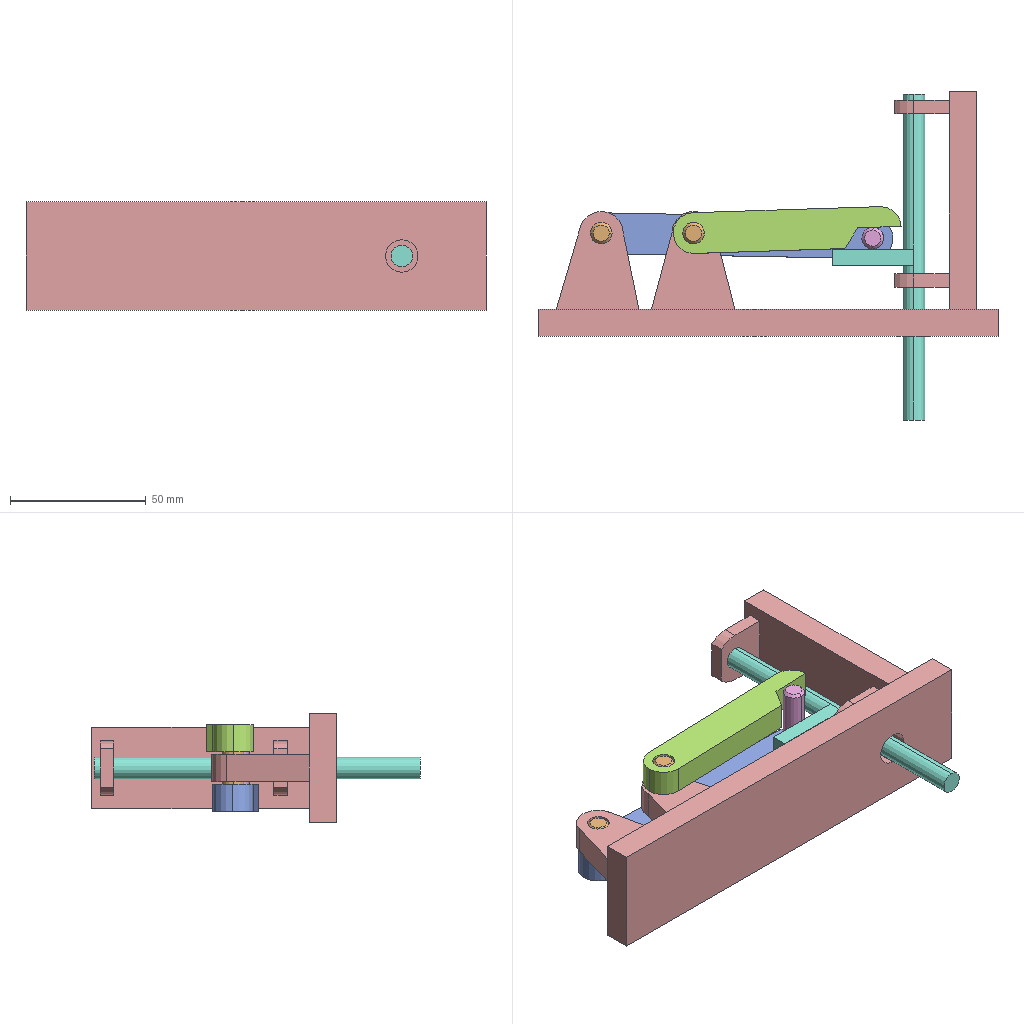Assembly | SolidWorks | 6 different items | 7 placed | box 169 x 121 x 40 mm
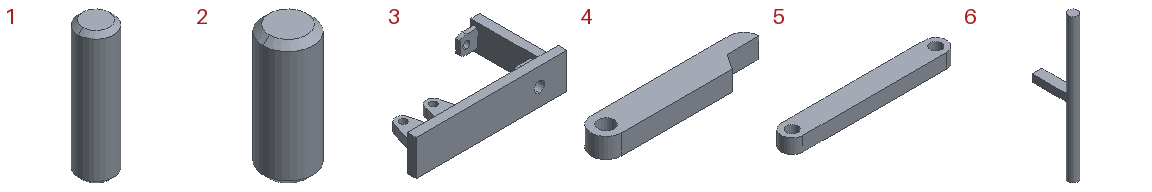Parts list (item | quantity | size | volume | features):
1 | x1 | 8 x 8 x 30 mm | 1485 mm3 | features Chamfer 1, Extrusion 1
2 | x2 | 8 x 8 x 20 mm | 982.271 mm3 | features Chamfer 1, Extrusion 1
3 | x1 | 169.404 x 90 x 40 mm | 108140 mm3 | features ICE 5, Extrusion 1
4 | x1 | 84 x 15 x 10 mm | 10349 mm3 | features Extrusion 1
5 | x1 | 115 x 15 x 10 mm | 15762 mm3 | features Extrusion 1
6 | x1 | 8 x 34 x 120 mm | 7321 mm3 | features Extrusion 1, ICE 1
Mates (type | each side: item.copy, entity, surface, feature):
Concentric | 3.1 face cylinder Boss-Extrude1 | 5.1 face cylinder Boss-Extrude1
DistanceDim | 5.1 face plane Boss-Extrude1 | 3.1 face plane Boss-Extrude1
Concentric | 3.1 face cylinder Boss-Extrude1 | 4.1 face cylinder Boss-Extrude1
DistanceDim | 4.1 face plane Boss-Extrude1 | 3.1 face plane Boss-Extrude1
Concentric | 5.1 face cylinder Boss-Extrude1 | 1.1 face cylinder Boss-Extrude1
Coincident | 4.1 face plane Boss-Extrude1 | 1.1 face plane Boss-Extrude1
Tangent | 4.1 face plane Boss-Extrude1 | 1.1 face cylinder Boss-Extrude1
Concentric | 3.1 face cylinder Cut-Extrude1 | 6.1 face cylinder Boss-Extrude1
Parallel | 3.1 face plane Boss-Extrude3 | 6.1 face plane Boss-Extrude2
Tangent | 1.1 face cylinder Boss-Extrude1 | 6.1 face plane Boss-Extrude2
Concentric | 3.1 face cylinder Boss-Extrude1 | 2.1 face cylinder Boss-Extrude1
Coincident | 3.1 face plane Boss-Extrude1 | 2.1 face plane Boss-Extrude1
Concentric | 4.1 face cylinder Boss-Extrude1 | 2.2 face cylinder Boss-Extrude1
Coincident | 4.1 face plane Boss-Extrude1 | 2.2 face plane Boss-Extrude1